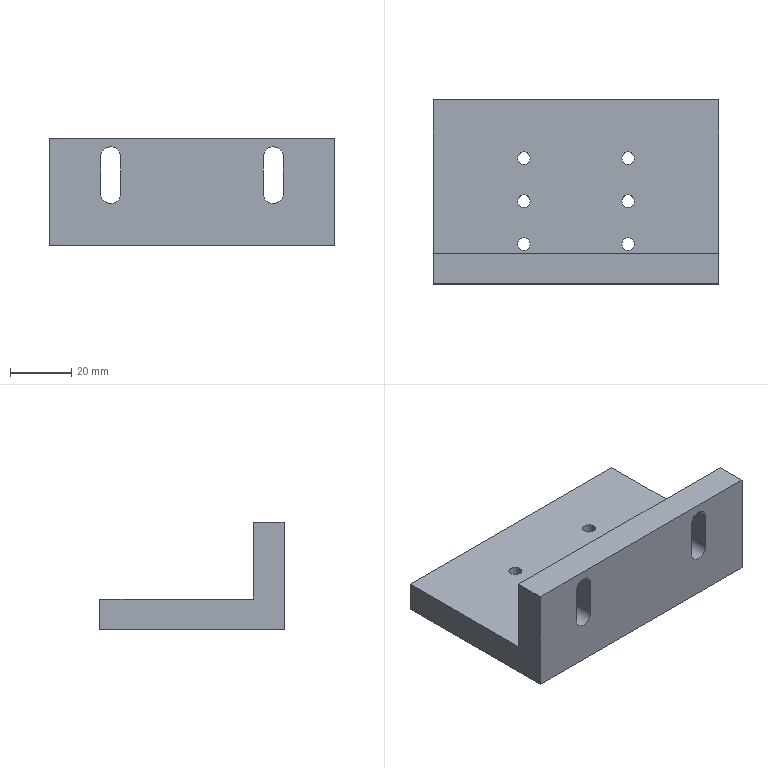Part | NX | 1 solid | 22 faces | box 93 x 60 x 35 mm | volume 76021 mm3 | plane 12 | cylinder 10 | commonest cylinder face diameters 4.134 x6 6.5 x4
STEP:
#1=CARTESIAN_POINT('',(-14.933,-3.,0.));
#2=VERTEX_POINT('',#1);
#3=CARTESIAN_POINT('',(-17.,-3.,0.));
#4=DIRECTION('',(0.,0.,1.));
#5=DIRECTION('',(1.,0.,0.));
#6=AXIS2_PLACEMENT_3D('',#3,#4,#5);
#7=CIRCLE('',#6,2.067);
#8=EDGE_CURVE('',#2,#2,#7,.T.);
#9=ORIENTED_EDGE('',*,*,#8,.T.);
#10=EDGE_LOOP('',(#9));
#11=FACE_BOUND('',#10,.T.);
#12=CARTESIAN_POINT('',(19.067,-3.,0.));
#13=VERTEX_POINT('',#12);
#14=CARTESIAN_POINT('',(17.,-3.,0.));
#15=DIRECTION('',(0.,0.,1.));
#16=DIRECTION('',(1.,0.,0.));
#17=AXIS2_PLACEMENT_3D('',#14,#15,#16);
#18=CIRCLE('',#17,2.067);
#19=EDGE_CURVE('',#13,#13,#18,.T.);
#20=ORIENTED_EDGE('',*,*,#19,.T.);
#21=EDGE_LOOP('',(#20));
#22=FACE_BOUND('',#21,.T.);
#23=CARTESIAN_POINT('',(-14.933,11.,0.));
#24=VERTEX_POINT('',#23);
#25=CARTESIAN_POINT('',(-17.,11.,0.));
#26=DIRECTION('',(0.,0.,1.));
#27=DIRECTION('',(1.,0.,0.));
#28=AXIS2_PLACEMENT_3D('',#25,#26,#27);
#29=CIRCLE('',#28,2.067);
#30=EDGE_CURVE('',#24,#24,#29,.T.);
#31=ORIENTED_EDGE('',*,*,#30,.T.);
#32=EDGE_LOOP('',(#31));
#33=FACE_BOUND('',#32,.T.);
#34=CARTESIAN_POINT('',(19.067,11.,0.));
#35=VERTEX_POINT('',#34);
#36=CARTESIAN_POINT('',(17.,11.,0.));
#37=DIRECTION('',(0.,0.,1.));
#38=DIRECTION('',(1.,0.,0.));
#39=AXIS2_PLACEMENT_3D('',#36,#37,#38);
#40=CIRCLE('',#39,2.067);
#41=EDGE_CURVE('',#35,#35,#40,.T.);
#42=ORIENTED_EDGE('',*,*,#41,.T.);
#43=EDGE_LOOP('',(#42));
#44=FACE_BOUND('',#43,.T.);
#45=CARTESIAN_POINT('',(-14.933,-17.,0.));
#46=VERTEX_POINT('',#45);
#47=CARTESIAN_POINT('',(-17.,-17.,0.));
#48=DIRECTION('',(0.,0.,1.));
#49=DIRECTION('',(1.,0.,0.));
#50=AXIS2_PLACEMENT_3D('',#47,#48,#49);
#51=CIRCLE('',#50,2.067);
#52=EDGE_CURVE('',#46,#46,#51,.T.);
#53=ORIENTED_EDGE('',*,*,#52,.T.);
#54=EDGE_LOOP('',(#53));
#55=FACE_BOUND('',#54,.T.);
#56=CARTESIAN_POINT('',(19.067,-17.,0.));
#57=VERTEX_POINT('',#56);
#58=CARTESIAN_POINT('',(17.,-17.,0.));
#59=DIRECTION('',(0.,0.,1.));
#60=DIRECTION('',(1.,0.,0.));
#61=AXIS2_PLACEMENT_3D('',#58,#59,#60);
#62=CIRCLE('',#61,2.067);
#63=EDGE_CURVE('',#57,#57,#62,.T.);
#64=ORIENTED_EDGE('',*,*,#63,.T.);
#65=EDGE_LOOP('',(#64));
#66=FACE_BOUND('',#65,.T.);
#67=CARTESIAN_POINT('',(46.5,-30.,0.));
#68=VERTEX_POINT('',#67);
#69=CARTESIAN_POINT('',(46.5,30.,0.));
#70=VERTEX_POINT('',#69);
#71=CARTESIAN_POINT('',(46.5,-30.,0.));
#72=DIRECTION('',(0.,1.,0.));
#73=VECTOR('',#72,1000.);
#74=LINE('',#71,#73);
#75=EDGE_CURVE('',#68,#70,#74,.T.);
#76=ORIENTED_EDGE('',*,*,#75,.F.);
#77=CARTESIAN_POINT('',(-46.5,-30.,0.));
#78=VERTEX_POINT('',#77);
#79=CARTESIAN_POINT('',(-46.5,-30.,0.));
#80=DIRECTION('',(1.,0.,0.));
#81=VECTOR('',#80,1000.);
#82=LINE('',#79,#81);
#83=EDGE_CURVE('',#78,#68,#82,.T.);
#84=ORIENTED_EDGE('',*,*,#83,.F.);
#85=CARTESIAN_POINT('',(-46.5,30.,0.));
#86=VERTEX_POINT('',#85);
#87=CARTESIAN_POINT('',(-46.5,30.,0.));
#88=DIRECTION('',(0.,-1.,0.));
#89=VECTOR('',#88,1000.);
#90=LINE('',#87,#89);
#91=EDGE_CURVE('',#86,#78,#90,.T.);
#92=ORIENTED_EDGE('',*,*,#91,.F.);
#93=CARTESIAN_POINT('',(46.5,30.,0.));
#94=DIRECTION('',(-1.,0.,0.));
#95=VECTOR('',#94,1000.);
#96=LINE('',#93,#95);
#97=EDGE_CURVE('',#70,#86,#96,.T.);
#98=ORIENTED_EDGE('',*,*,#97,.F.);
#99=EDGE_LOOP('',(#76,#84,#92,#98));
#100=FACE_BOUND('',#99,.T.);
#101=CARTESIAN_POINT('',(0.,0.,0.));
#102=DIRECTION('',(0.,0.,1.));
#103=DIRECTION('',(1.,0.,0.));
#104=AXIS2_PLACEMENT_3D('',#101,#102,#103);
#105=PLANE('',#104);
#106=ADVANCED_FACE('',(#11,#22,#33,#44,#55,#66,#100),#105,.F.);
#107=ORIENTED_EDGE('',*,*,#75,.T.);
#108=CARTESIAN_POINT('',(46.5,30.,10.));
#109=VERTEX_POINT('',#108);
#110=CARTESIAN_POINT('',(46.5,30.,0.));
#111=DIRECTION('',(0.,0.,1.));
#112=VECTOR('',#111,1000.);
#113=LINE('',#110,#112);
#114=EDGE_CURVE('',#70,#109,#113,.T.);
#115=ORIENTED_EDGE('',*,*,#114,.T.);
#116=CARTESIAN_POINT('',(46.5,-20.,10.));
#117=VERTEX_POINT('',#116);
#118=CARTESIAN_POINT('',(46.5,-30.,10.));
#119=DIRECTION('',(0.,1.,0.));
#120=VECTOR('',#119,1000.);
#121=LINE('',#118,#120);
#122=EDGE_CURVE('',#117,#109,#121,.T.);
#123=ORIENTED_EDGE('',*,*,#122,.F.);
#124=CARTESIAN_POINT('',(46.5,-20.,35.));
#125=VERTEX_POINT('',#124);
#126=CARTESIAN_POINT('',(46.5,-20.,10.));
#127=DIRECTION('',(0.,0.,1.));
#128=VECTOR('',#127,1000.);
#129=LINE('',#126,#128);
#130=EDGE_CURVE('',#117,#125,#129,.T.);
#131=ORIENTED_EDGE('',*,*,#130,.T.);
#132=CARTESIAN_POINT('',(46.5,-30.,35.));
#133=VERTEX_POINT('',#132);
#134=CARTESIAN_POINT('',(46.5,-30.,35.));
#135=DIRECTION('',(0.,1.,0.));
#136=VECTOR('',#135,1000.);
#137=LINE('',#134,#136);
#138=EDGE_CURVE('',#133,#125,#137,.T.);
#139=ORIENTED_EDGE('',*,*,#138,.F.);
#140=CARTESIAN_POINT('',(46.5,-30.,0.));
#141=DIRECTION('',(0.,0.,1.));
#142=VECTOR('',#141,1000.);
#143=LINE('',#140,#142);
#144=EDGE_CURVE('',#68,#133,#143,.T.);
#145=ORIENTED_EDGE('',*,*,#144,.F.);
#146=EDGE_LOOP('',(#107,#115,#123,#131,#139,#145));
#147=FACE_BOUND('',#146,.T.);
#148=CARTESIAN_POINT('',(46.5,-30.,0.));
#149=DIRECTION('',(1.,0.,0.));
#150=DIRECTION('',(0.,1.,0.));
#151=AXIS2_PLACEMENT_3D('',#148,#149,#150);
#152=PLANE('',#151);
#153=ADVANCED_FACE('',(#147),#152,.T.);
#154=ORIENTED_EDGE('',*,*,#97,.T.);
#155=CARTESIAN_POINT('',(-46.5,30.,10.));
#156=VERTEX_POINT('',#155);
#157=CARTESIAN_POINT('',(-46.5,30.,0.));
#158=DIRECTION('',(0.,0.,1.));
#159=VECTOR('',#158,1000.);
#160=LINE('',#157,#159);
#161=EDGE_CURVE('',#86,#156,#160,.T.);
#162=ORIENTED_EDGE('',*,*,#161,.T.);
#163=CARTESIAN_POINT('',(46.5,30.,10.));
#164=DIRECTION('',(-1.,0.,0.));
#165=VECTOR('',#164,1000.);
#166=LINE('',#163,#165);
#167=EDGE_CURVE('',#109,#156,#166,.T.);
#168=ORIENTED_EDGE('',*,*,#167,.F.);
#169=ORIENTED_EDGE('',*,*,#114,.F.);
#170=EDGE_LOOP('',(#154,#162,#168,#169));
#171=FACE_BOUND('',#170,.T.);
#172=CARTESIAN_POINT('',(46.5,30.,0.));
#173=DIRECTION('',(0.,1.,0.));
#174=DIRECTION('',(-1.,0.,0.));
#175=AXIS2_PLACEMENT_3D('',#172,#173,#174);
#176=PLANE('',#175);
#177=ADVANCED_FACE('',(#171),#176,.T.);
#178=ORIENTED_EDGE('',*,*,#91,.T.);
#179=CARTESIAN_POINT('',(-46.5,-30.,35.));
#180=VERTEX_POINT('',#179);
#181=CARTESIAN_POINT('',(-46.5,-30.,0.));
#182=DIRECTION('',(0.,0.,1.));
#183=VECTOR('',#182,1000.);
#184=LINE('',#181,#183);
#185=EDGE_CURVE('',#78,#180,#184,.T.);
#186=ORIENTED_EDGE('',*,*,#185,.T.);
#187=CARTESIAN_POINT('',(-46.5,-20.,35.));
#188=VERTEX_POINT('',#187);
#189=CARTESIAN_POINT('',(-46.5,30.,35.));
#190=DIRECTION('',(0.,-1.,0.));
#191=VECTOR('',#190,1000.);
#192=LINE('',#189,#191);
#193=EDGE_CURVE('',#188,#180,#192,.T.);
#194=ORIENTED_EDGE('',*,*,#193,.F.);
#195=CARTESIAN_POINT('',(-46.5,-20.,10.));
#196=VERTEX_POINT('',#195);
#197=CARTESIAN_POINT('',(-46.5,-20.,10.));
#198=DIRECTION('',(0.,0.,1.));
#199=VECTOR('',#198,1000.);
#200=LINE('',#197,#199);
#201=EDGE_CURVE('',#196,#188,#200,.T.);
#202=ORIENTED_EDGE('',*,*,#201,.F.);
#203=CARTESIAN_POINT('',(-46.5,30.,10.));
#204=DIRECTION('',(0.,-1.,0.));
#205=VECTOR('',#204,1000.);
#206=LINE('',#203,#205);
#207=EDGE_CURVE('',#156,#196,#206,.T.);
#208=ORIENTED_EDGE('',*,*,#207,.F.);
#209=ORIENTED_EDGE('',*,*,#161,.F.);
#210=EDGE_LOOP('',(#178,#186,#194,#202,#208,#209));
#211=FACE_BOUND('',#210,.T.);
#212=CARTESIAN_POINT('',(-46.5,30.,0.));
#213=DIRECTION('',(-1.,0.,0.));
#214=DIRECTION('',(0.,-1.,0.));
#215=AXIS2_PLACEMENT_3D('',#212,#213,#214);
#216=PLANE('',#215);
#217=ADVANCED_FACE('',(#211),#216,.T.);
#218=CARTESIAN_POINT('',(-29.75,-30.,17.));
#219=VERTEX_POINT('',#218);
#220=CARTESIAN_POINT('',(-29.75,-30.,29.));
#221=VERTEX_POINT('',#220);
#222=CARTESIAN_POINT('',(-29.75,-30.,14.5));
#223=DIRECTION('',(0.,0.,1.));
#224=VECTOR('',#223,1000.);
#225=LINE('',#222,#224);
#226=EDGE_CURVE('',#219,#221,#225,.T.);
#227=ORIENTED_EDGE('',*,*,#226,.T.);
#228=CARTESIAN_POINT('',(-23.25,-30.,29.));
#229=VERTEX_POINT('',#228);
#230=CARTESIAN_POINT('',(-26.5,-30.,29.));
#231=DIRECTION('',(0.,1.,0.));
#232=DIRECTION('',(-1.,0.,0.));
#233=AXIS2_PLACEMENT_3D('',#230,#231,#232);
#234=CIRCLE('',#233,3.25);
#235=EDGE_CURVE('',#221,#229,#234,.T.);
#236=ORIENTED_EDGE('',*,*,#235,.T.);
#237=CARTESIAN_POINT('',(-23.25,-30.,17.));
#238=VERTEX_POINT('',#237);
#239=CARTESIAN_POINT('',(-23.25,-30.,8.5));
#240=DIRECTION('',(0.,0.,-1.));
#241=VECTOR('',#240,1000.);
#242=LINE('',#239,#241);
#243=EDGE_CURVE('',#229,#238,#242,.T.);
#244=ORIENTED_EDGE('',*,*,#243,.T.);
#245=CARTESIAN_POINT('',(-26.5,-30.,17.));
#246=DIRECTION('',(0.,1.,0.));
#247=DIRECTION('',(1.,0.,0.));
#248=AXIS2_PLACEMENT_3D('',#245,#246,#247);
#249=CIRCLE('',#248,3.25);
#250=EDGE_CURVE('',#238,#219,#249,.T.);
#251=ORIENTED_EDGE('',*,*,#250,.T.);
#252=EDGE_LOOP('',(#227,#236,#244,#251));
#253=FACE_BOUND('',#252,.T.);
#254=CARTESIAN_POINT('',(23.25,-30.,17.));
#255=VERTEX_POINT('',#254);
#256=CARTESIAN_POINT('',(23.25,-30.,29.));
#257=VERTEX_POINT('',#256);
#258=CARTESIAN_POINT('',(23.25,-30.,14.5));
#259=DIRECTION('',(0.,0.,1.));
#260=VECTOR('',#259,1000.);
#261=LINE('',#258,#260);
#262=EDGE_CURVE('',#255,#257,#261,.T.);
#263=ORIENTED_EDGE('',*,*,#262,.T.);
#264=CARTESIAN_POINT('',(29.75,-30.,29.));
#265=VERTEX_POINT('',#264);
#266=CARTESIAN_POINT('',(26.5,-30.,29.));
#267=DIRECTION('',(0.,1.,0.));
#268=DIRECTION('',(-1.,0.,0.));
#269=AXIS2_PLACEMENT_3D('',#266,#267,#268);
#270=CIRCLE('',#269,3.25);
#271=EDGE_CURVE('',#257,#265,#270,.T.);
#272=ORIENTED_EDGE('',*,*,#271,.T.);
#273=CARTESIAN_POINT('',(29.75,-30.,17.));
#274=VERTEX_POINT('',#273);
#275=CARTESIAN_POINT('',(29.75,-30.,8.5));
#276=DIRECTION('',(0.,0.,-1.));
#277=VECTOR('',#276,1000.);
#278=LINE('',#275,#277);
#279=EDGE_CURVE('',#265,#274,#278,.T.);
#280=ORIENTED_EDGE('',*,*,#279,.T.);
#281=CARTESIAN_POINT('',(26.5,-30.,17.));
#282=DIRECTION('',(0.,1.,0.));
#283=DIRECTION('',(1.,0.,0.));
#284=AXIS2_PLACEMENT_3D('',#281,#282,#283);
#285=CIRCLE('',#284,3.25);
#286=EDGE_CURVE('',#274,#255,#285,.T.);
#287=ORIENTED_EDGE('',*,*,#286,.T.);
#288=EDGE_LOOP('',(#263,#272,#280,#287));
#289=FACE_BOUND('',#288,.T.);
#290=ORIENTED_EDGE('',*,*,#83,.T.);
#291=ORIENTED_EDGE('',*,*,#144,.T.);
#292=CARTESIAN_POINT('',(-46.5,-30.,35.));
#293=DIRECTION('',(1.,0.,0.));
#294=VECTOR('',#293,1000.);
#295=LINE('',#292,#294);
#296=EDGE_CURVE('',#180,#133,#295,.T.);
#297=ORIENTED_EDGE('',*,*,#296,.F.);
#298=ORIENTED_EDGE('',*,*,#185,.F.);
#299=EDGE_LOOP('',(#290,#291,#297,#298));
#300=FACE_BOUND('',#299,.T.);
#301=CARTESIAN_POINT('',(-46.5,-30.,0.));
#302=DIRECTION('',(0.,-1.,0.));
#303=DIRECTION('',(1.,0.,0.));
#304=AXIS2_PLACEMENT_3D('',#301,#302,#303);
#305=PLANE('',#304);
#306=ADVANCED_FACE('',(#253,#289,#300),#305,.T.);
#307=CARTESIAN_POINT('',(-14.933,-3.,10.));
#308=VERTEX_POINT('',#307);
#309=CARTESIAN_POINT('',(-17.,-3.,10.));
#310=DIRECTION('',(0.,0.,-1.));
#311=DIRECTION('',(1.,0.,0.));
#312=AXIS2_PLACEMENT_3D('',#309,#310,#311);
#313=CIRCLE('',#312,2.067);
#314=EDGE_CURVE('',#308,#308,#313,.T.);
#315=ORIENTED_EDGE('',*,*,#314,.T.);
#316=EDGE_LOOP('',(#315));
#317=FACE_BOUND('',#316,.T.);
#318=CARTESIAN_POINT('',(19.067,-3.,10.));
#319=VERTEX_POINT('',#318);
#320=CARTESIAN_POINT('',(17.,-3.,10.));
#321=DIRECTION('',(0.,0.,-1.));
#322=DIRECTION('',(1.,0.,0.));
#323=AXIS2_PLACEMENT_3D('',#320,#321,#322);
#324=CIRCLE('',#323,2.067);
#325=EDGE_CURVE('',#319,#319,#324,.T.);
#326=ORIENTED_EDGE('',*,*,#325,.T.);
#327=EDGE_LOOP('',(#326));
#328=FACE_BOUND('',#327,.T.);
#329=CARTESIAN_POINT('',(-14.933,11.,10.));
#330=VERTEX_POINT('',#329);
#331=CARTESIAN_POINT('',(-17.,11.,10.));
#332=DIRECTION('',(0.,0.,-1.));
#333=DIRECTION('',(1.,0.,0.));
#334=AXIS2_PLACEMENT_3D('',#331,#332,#333);
#335=CIRCLE('',#334,2.067);
#336=EDGE_CURVE('',#330,#330,#335,.T.);
#337=ORIENTED_EDGE('',*,*,#336,.T.);
#338=EDGE_LOOP('',(#337));
#339=FACE_BOUND('',#338,.T.);
#340=CARTESIAN_POINT('',(19.067,11.,10.));
#341=VERTEX_POINT('',#340);
#342=CARTESIAN_POINT('',(17.,11.,10.));
#343=DIRECTION('',(0.,0.,-1.));
#344=DIRECTION('',(1.,0.,0.));
#345=AXIS2_PLACEMENT_3D('',#342,#343,#344);
#346=CIRCLE('',#345,2.067);
#347=EDGE_CURVE('',#341,#341,#346,.T.);
#348=ORIENTED_EDGE('',*,*,#347,.T.);
#349=EDGE_LOOP('',(#348));
#350=FACE_BOUND('',#349,.T.);
#351=CARTESIAN_POINT('',(-14.933,-17.,10.));
#352=VERTEX_POINT('',#351);
#353=CARTESIAN_POINT('',(-17.,-17.,10.));
#354=DIRECTION('',(0.,0.,-1.));
#355=DIRECTION('',(1.,0.,0.));
#356=AXIS2_PLACEMENT_3D('',#353,#354,#355);
#357=CIRCLE('',#356,2.067);
#358=EDGE_CURVE('',#352,#352,#357,.T.);
#359=ORIENTED_EDGE('',*,*,#358,.T.);
#360=EDGE_LOOP('',(#359));
#361=FACE_BOUND('',#360,.T.);
#362=CARTESIAN_POINT('',(19.067,-17.,10.));
#363=VERTEX_POINT('',#362);
#364=CARTESIAN_POINT('',(17.,-17.,10.));
#365=DIRECTION('',(0.,0.,-1.));
#366=DIRECTION('',(1.,0.,0.));
#367=AXIS2_PLACEMENT_3D('',#364,#365,#366);
#368=CIRCLE('',#367,2.067);
#369=EDGE_CURVE('',#363,#363,#368,.T.);
#370=ORIENTED_EDGE('',*,*,#369,.T.);
#371=EDGE_LOOP('',(#370));
#372=FACE_BOUND('',#371,.T.);
#373=CARTESIAN_POINT('',(23.25,-20.,10.));
#374=DIRECTION('',(1.,0.,0.));
#375=VECTOR('',#374,1000.);
#376=LINE('',#373,#375);
#377=EDGE_CURVE('',#196,#117,#376,.T.);
#378=ORIENTED_EDGE('',*,*,#377,.T.);
#379=ORIENTED_EDGE('',*,*,#122,.T.);
#380=ORIENTED_EDGE('',*,*,#167,.T.);
#381=ORIENTED_EDGE('',*,*,#207,.T.);
#382=EDGE_LOOP('',(#378,#379,#380,#381));
#383=FACE_BOUND('',#382,.T.);
#384=CARTESIAN_POINT('',(0.,0.,10.));
#385=DIRECTION('',(0.,0.,1.));
#386=DIRECTION('',(1.,0.,0.));
#387=AXIS2_PLACEMENT_3D('',#384,#385,#386);
#388=PLANE('',#387);
#389=ADVANCED_FACE('',(#317,#328,#339,#350,#361,#372,#383),#388,.T.);
#390=ORIENTED_EDGE('',*,*,#138,.T.);
#391=CARTESIAN_POINT('',(46.5,-20.,35.));
#392=DIRECTION('',(-1.,0.,0.));
#393=VECTOR('',#392,1000.);
#394=LINE('',#391,#393);
#395=EDGE_CURVE('',#125,#188,#394,.T.);
#396=ORIENTED_EDGE('',*,*,#395,.T.);
#397=ORIENTED_EDGE('',*,*,#193,.T.);
#398=ORIENTED_EDGE('',*,*,#296,.T.);
#399=EDGE_LOOP('',(#390,#396,#397,#398));
#400=FACE_BOUND('',#399,.T.);
#401=CARTESIAN_POINT('',(0.,-25.,35.));
#402=DIRECTION('',(0.,0.,1.));
#403=DIRECTION('',(1.,0.,0.));
#404=AXIS2_PLACEMENT_3D('',#401,#402,#403);
#405=PLANE('',#404);
#406=ADVANCED_FACE('',(#400),#405,.T.);
#407=CARTESIAN_POINT('',(-29.75,-20.,29.));
#408=VERTEX_POINT('',#407);
#409=CARTESIAN_POINT('',(-29.75,-20.,17.));
#410=VERTEX_POINT('',#409);
#411=CARTESIAN_POINT('',(-29.75,-20.,19.5));
#412=DIRECTION('',(0.,0.,-1.));
#413=VECTOR('',#412,1000.);
#414=LINE('',#411,#413);
#415=EDGE_CURVE('',#408,#410,#414,.T.);
#416=ORIENTED_EDGE('',*,*,#415,.T.);
#417=CARTESIAN_POINT('',(-23.25,-20.,17.));
#418=VERTEX_POINT('',#417);
#419=CARTESIAN_POINT('',(-26.5,-20.,17.));
#420=DIRECTION('',(0.,-1.,0.));
#421=DIRECTION('',(1.,0.,0.));
#422=AXIS2_PLACEMENT_3D('',#419,#420,#421);
#423=CIRCLE('',#422,3.25);
#424=EDGE_CURVE('',#410,#418,#423,.T.);
#425=ORIENTED_EDGE('',*,*,#424,.T.);
#426=CARTESIAN_POINT('',(-23.25,-20.,29.));
#427=VERTEX_POINT('',#426);
#428=CARTESIAN_POINT('',(-23.25,-20.,13.5));
#429=DIRECTION('',(0.,0.,1.));
#430=VECTOR('',#429,1000.);
#431=LINE('',#428,#430);
#432=EDGE_CURVE('',#418,#427,#431,.T.);
#433=ORIENTED_EDGE('',*,*,#432,.T.);
#434=CARTESIAN_POINT('',(-26.5,-20.,29.));
#435=DIRECTION('',(0.,-1.,0.));
#436=DIRECTION('',(-1.,0.,0.));
#437=AXIS2_PLACEMENT_3D('',#434,#435,#436);
#438=CIRCLE('',#437,3.25);
#439=EDGE_CURVE('',#427,#408,#438,.T.);
#440=ORIENTED_EDGE('',*,*,#439,.T.);
#441=EDGE_LOOP('',(#416,#425,#433,#440));
#442=FACE_BOUND('',#441,.T.);
#443=CARTESIAN_POINT('',(23.25,-20.,29.));
#444=VERTEX_POINT('',#443);
#445=CARTESIAN_POINT('',(23.25,-20.,17.));
#446=VERTEX_POINT('',#445);
#447=CARTESIAN_POINT('',(23.25,-20.,19.5));
#448=DIRECTION('',(0.,0.,-1.));
#449=VECTOR('',#448,1000.);
#450=LINE('',#447,#449);
#451=EDGE_CURVE('',#444,#446,#450,.T.);
#452=ORIENTED_EDGE('',*,*,#451,.T.);
#453=CARTESIAN_POINT('',(29.75,-20.,17.));
#454=VERTEX_POINT('',#453);
#455=CARTESIAN_POINT('',(26.5,-20.,17.));
#456=DIRECTION('',(0.,-1.,0.));
#457=DIRECTION('',(1.,0.,0.));
#458=AXIS2_PLACEMENT_3D('',#455,#456,#457);
#459=CIRCLE('',#458,3.25);
#460=EDGE_CURVE('',#446,#454,#459,.T.);
#461=ORIENTED_EDGE('',*,*,#460,.T.);
#462=CARTESIAN_POINT('',(29.75,-20.,29.));
#463=VERTEX_POINT('',#462);
#464=CARTESIAN_POINT('',(29.75,-20.,13.5));
#465=DIRECTION('',(0.,0.,1.));
#466=VECTOR('',#465,1000.);
#467=LINE('',#464,#466);
#468=EDGE_CURVE('',#454,#463,#467,.T.);
#469=ORIENTED_EDGE('',*,*,#468,.T.);
#470=CARTESIAN_POINT('',(26.5,-20.,29.));
#471=DIRECTION('',(0.,-1.,0.));
#472=DIRECTION('',(-1.,0.,0.));
#473=AXIS2_PLACEMENT_3D('',#470,#471,#472);
#474=CIRCLE('',#473,3.25);
#475=EDGE_CURVE('',#463,#444,#474,.T.);
#476=ORIENTED_EDGE('',*,*,#475,.T.);
#477=EDGE_LOOP('',(#452,#461,#469,#476));
#478=FACE_BOUND('',#477,.T.);
#479=ORIENTED_EDGE('',*,*,#377,.F.);
#480=ORIENTED_EDGE('',*,*,#201,.T.);
#481=ORIENTED_EDGE('',*,*,#395,.F.);
#482=ORIENTED_EDGE('',*,*,#130,.F.);
#483=EDGE_LOOP('',(#479,#480,#481,#482));
#484=FACE_BOUND('',#483,.T.);
#485=CARTESIAN_POINT('',(46.5,-20.,10.));
#486=DIRECTION('',(0.,1.,0.));
#487=DIRECTION('',(-1.,0.,0.));
#488=AXIS2_PLACEMENT_3D('',#485,#486,#487);
#489=PLANE('',#488);
#490=ADVANCED_FACE('',(#442,#478,#484),#489,.T.);
#491=ORIENTED_EDGE('',*,*,#8,.F.);
#492=EDGE_LOOP('',(#491));
#493=FACE_BOUND('',#492,.T.);
#494=ORIENTED_EDGE('',*,*,#314,.F.);
#495=EDGE_LOOP('',(#494));
#496=FACE_BOUND('',#495,.T.);
#497=CARTESIAN_POINT('',(-17.,-3.,-106.078));
#498=DIRECTION('',(0.,0.,1.));
#499=DIRECTION('',(1.,0.,0.));
#500=AXIS2_PLACEMENT_3D('',#497,#498,#499);
#501=CYLINDRICAL_SURFACE('',#500,2.067);
#502=ADVANCED_FACE('',(#493,#496),#501,.F.);
#503=ORIENTED_EDGE('',*,*,#19,.F.);
#504=EDGE_LOOP('',(#503));
#505=FACE_BOUND('',#504,.T.);
#506=ORIENTED_EDGE('',*,*,#325,.F.);
#507=EDGE_LOOP('',(#506));
#508=FACE_BOUND('',#507,.T.);
#509=CARTESIAN_POINT('',(17.,-3.,-106.078));
#510=DIRECTION('',(0.,0.,1.));
#511=DIRECTION('',(1.,0.,0.));
#512=AXIS2_PLACEMENT_3D('',#509,#510,#511);
#513=CYLINDRICAL_SURFACE('',#512,2.067);
#514=ADVANCED_FACE('',(#505,#508),#513,.F.);
#515=ORIENTED_EDGE('',*,*,#30,.F.);
#516=EDGE_LOOP('',(#515));
#517=FACE_BOUND('',#516,.T.);
#518=ORIENTED_EDGE('',*,*,#336,.F.);
#519=EDGE_LOOP('',(#518));
#520=FACE_BOUND('',#519,.T.);
#521=CARTESIAN_POINT('',(-17.,11.,-106.078));
#522=DIRECTION('',(0.,0.,1.));
#523=DIRECTION('',(1.,0.,0.));
#524=AXIS2_PLACEMENT_3D('',#521,#522,#523);
#525=CYLINDRICAL_SURFACE('',#524,2.067);
#526=ADVANCED_FACE('',(#517,#520),#525,.F.);
#527=ORIENTED_EDGE('',*,*,#41,.F.);
#528=EDGE_LOOP('',(#527));
#529=FACE_BOUND('',#528,.T.);
#530=ORIENTED_EDGE('',*,*,#347,.F.);
#531=EDGE_LOOP('',(#530));
#532=FACE_BOUND('',#531,.T.);
#533=CARTESIAN_POINT('',(17.,11.,-106.078));
#534=DIRECTION('',(0.,0.,1.));
#535=DIRECTION('',(1.,0.,0.));
#536=AXIS2_PLACEMENT_3D('',#533,#534,#535);
#537=CYLINDRICAL_SURFACE('',#536,2.067);
#538=ADVANCED_FACE('',(#529,#532),#537,.F.);
#539=ORIENTED_EDGE('',*,*,#52,.F.);
#540=EDGE_LOOP('',(#539));
#541=FACE_BOUND('',#540,.T.);
#542=ORIENTED_EDGE('',*,*,#358,.F.);
#543=EDGE_LOOP('',(#542));
#544=FACE_BOUND('',#543,.T.);
#545=CARTESIAN_POINT('',(-17.,-17.,-106.078));
#546=DIRECTION('',(0.,0.,1.));
#547=DIRECTION('',(1.,0.,0.));
#548=AXIS2_PLACEMENT_3D('',#545,#546,#547);
#549=CYLINDRICAL_SURFACE('',#548,2.067);
#550=ADVANCED_FACE('',(#541,#544),#549,.F.);
#551=ORIENTED_EDGE('',*,*,#63,.F.);
#552=EDGE_LOOP('',(#551));
#553=FACE_BOUND('',#552,.T.);
#554=ORIENTED_EDGE('',*,*,#369,.F.);
#555=EDGE_LOOP('',(#554));
#556=FACE_BOUND('',#555,.T.);
#557=CARTESIAN_POINT('',(17.,-17.,-106.078));
#558=DIRECTION('',(0.,0.,1.));
#559=DIRECTION('',(1.,0.,0.));
#560=AXIS2_PLACEMENT_3D('',#557,#558,#559);
#561=CYLINDRICAL_SURFACE('',#560,2.067);
#562=ADVANCED_FACE('',(#553,#556),#561,.F.);
#563=ORIENTED_EDGE('',*,*,#235,.F.);
#564=CARTESIAN_POINT('',(-29.75,-20.,29.));
#565=DIRECTION('',(0.,-1.,0.));
#566=VECTOR('',#565,1000.);
#567=LINE('',#564,#566);
#568=EDGE_CURVE('',#408,#221,#567,.T.);
#569=ORIENTED_EDGE('',*,*,#568,.F.);
#570=ORIENTED_EDGE('',*,*,#439,.F.);
#571=CARTESIAN_POINT('',(-23.25,-20.,29.));
#572=DIRECTION('',(0.,-1.,0.));
#573=VECTOR('',#572,1000.);
#574=LINE('',#571,#573);
#575=EDGE_CURVE('',#427,#229,#574,.T.);
#576=ORIENTED_EDGE('',*,*,#575,.T.);
#577=EDGE_LOOP('',(#563,#569,#570,#576));
#578=FACE_BOUND('',#577,.T.);
#579=CARTESIAN_POINT('',(-26.5,-20.,29.));
#580=DIRECTION('',(0.,-1.,0.));
#581=DIRECTION('',(-1.,0.,0.));
#582=AXIS2_PLACEMENT_3D('',#579,#580,#581);
#583=CYLINDRICAL_SURFACE('',#582,3.25);
#584=ADVANCED_FACE('',(#578),#583,.F.);
#585=ORIENTED_EDGE('',*,*,#226,.F.);
#586=CARTESIAN_POINT('',(-29.75,-20.,17.));
#587=DIRECTION('',(0.,-1.,0.));
#588=VECTOR('',#587,1000.);
#589=LINE('',#586,#588);
#590=EDGE_CURVE('',#410,#219,#589,.T.);
#591=ORIENTED_EDGE('',*,*,#590,.F.);
#592=ORIENTED_EDGE('',*,*,#415,.F.);
#593=ORIENTED_EDGE('',*,*,#568,.T.);
#594=EDGE_LOOP('',(#585,#591,#592,#593));
#595=FACE_BOUND('',#594,.T.);
#596=CARTESIAN_POINT('',(-29.75,-20.,29.));
#597=DIRECTION('',(-1.,0.,0.));
#598=DIRECTION('',(0.,0.,-1.));
#599=AXIS2_PLACEMENT_3D('',#596,#597,#598);
#600=PLANE('',#599);
#601=ADVANCED_FACE('',(#595),#600,.F.);
#602=ORIENTED_EDGE('',*,*,#250,.F.);
#603=CARTESIAN_POINT('',(-23.25,-20.,17.));
#604=DIRECTION('',(0.,-1.,0.));
#605=VECTOR('',#604,1000.);
#606=LINE('',#603,#605);
#607=EDGE_CURVE('',#418,#238,#606,.T.);
#608=ORIENTED_EDGE('',*,*,#607,.F.);
#609=ORIENTED_EDGE('',*,*,#424,.F.);
#610=ORIENTED_EDGE('',*,*,#590,.T.);
#611=EDGE_LOOP('',(#602,#608,#609,#610));
#612=FACE_BOUND('',#611,.T.);
#613=CARTESIAN_POINT('',(-26.5,-20.,17.));
#614=DIRECTION('',(0.,-1.,0.));
#615=DIRECTION('',(1.,0.,0.));
#616=AXIS2_PLACEMENT_3D('',#613,#614,#615);
#617=CYLINDRICAL_SURFACE('',#616,3.25);
#618=ADVANCED_FACE('',(#612),#617,.F.);
#619=ORIENTED_EDGE('',*,*,#243,.F.);
#620=ORIENTED_EDGE('',*,*,#575,.F.);
#621=ORIENTED_EDGE('',*,*,#432,.F.);
#622=ORIENTED_EDGE('',*,*,#607,.T.);
#623=EDGE_LOOP('',(#619,#620,#621,#622));
#624=FACE_BOUND('',#623,.T.);
#625=CARTESIAN_POINT('',(-23.25,-20.,17.));
#626=DIRECTION('',(1.,0.,0.));
#627=DIRECTION('',(0.,0.,1.));
#628=AXIS2_PLACEMENT_3D('',#625,#626,#627);
#629=PLANE('',#628);
#630=ADVANCED_FACE('',(#624),#629,.F.);
#631=ORIENTED_EDGE('',*,*,#271,.F.);
#632=CARTESIAN_POINT('',(23.25,-20.,29.));
#633=DIRECTION('',(0.,-1.,0.));
#634=VECTOR('',#633,1000.);
#635=LINE('',#632,#634);
#636=EDGE_CURVE('',#444,#257,#635,.T.);
#637=ORIENTED_EDGE('',*,*,#636,.F.);
#638=ORIENTED_EDGE('',*,*,#475,.F.);
#639=CARTESIAN_POINT('',(29.75,-20.,29.));
#640=DIRECTION('',(0.,-1.,0.));
#641=VECTOR('',#640,1000.);
#642=LINE('',#639,#641);
#643=EDGE_CURVE('',#463,#265,#642,.T.);
#644=ORIENTED_EDGE('',*,*,#643,.T.);
#645=EDGE_LOOP('',(#631,#637,#638,#644));
#646=FACE_BOUND('',#645,.T.);
#647=CARTESIAN_POINT('',(26.5,-20.,29.));
#648=DIRECTION('',(0.,-1.,0.));
#649=DIRECTION('',(-1.,0.,0.));
#650=AXIS2_PLACEMENT_3D('',#647,#648,#649);
#651=CYLINDRICAL_SURFACE('',#650,3.25);
#652=ADVANCED_FACE('',(#646),#651,.F.);
#653=ORIENTED_EDGE('',*,*,#262,.F.);
#654=CARTESIAN_POINT('',(23.25,-20.,17.));
#655=DIRECTION('',(0.,-1.,0.));
#656=VECTOR('',#655,1000.);
#657=LINE('',#654,#656);
#658=EDGE_CURVE('',#446,#255,#657,.T.);
#659=ORIENTED_EDGE('',*,*,#658,.F.);
#660=ORIENTED_EDGE('',*,*,#451,.F.);
#661=ORIENTED_EDGE('',*,*,#636,.T.);
#662=EDGE_LOOP('',(#653,#659,#660,#661));
#663=FACE_BOUND('',#662,.T.);
#664=CARTESIAN_POINT('',(23.25,-20.,29.));
#665=DIRECTION('',(-1.,0.,0.));
#666=DIRECTION('',(0.,0.,-1.));
#667=AXIS2_PLACEMENT_3D('',#664,#665,#666);
#668=PLANE('',#667);
#669=ADVANCED_FACE('',(#663),#668,.F.);
#670=ORIENTED_EDGE('',*,*,#286,.F.);
#671=CARTESIAN_POINT('',(29.75,-20.,17.));
#672=DIRECTION('',(0.,-1.,0.));
#673=VECTOR('',#672,1000.);
#674=LINE('',#671,#673);
#675=EDGE_CURVE('',#454,#274,#674,.T.);
#676=ORIENTED_EDGE('',*,*,#675,.F.);
#677=ORIENTED_EDGE('',*,*,#460,.F.);
#678=ORIENTED_EDGE('',*,*,#658,.T.);
#679=EDGE_LOOP('',(#670,#676,#677,#678));
#680=FACE_BOUND('',#679,.T.);
#681=CARTESIAN_POINT('',(26.5,-20.,17.));
#682=DIRECTION('',(0.,-1.,0.));
#683=DIRECTION('',(1.,0.,0.));
#684=AXIS2_PLACEMENT_3D('',#681,#682,#683);
#685=CYLINDRICAL_SURFACE('',#684,3.25);
#686=ADVANCED_FACE('',(#680),#685,.F.);
#687=ORIENTED_EDGE('',*,*,#279,.F.);
#688=ORIENTED_EDGE('',*,*,#643,.F.);
#689=ORIENTED_EDGE('',*,*,#468,.F.);
#690=ORIENTED_EDGE('',*,*,#675,.T.);
#691=EDGE_LOOP('',(#687,#688,#689,#690));
#692=FACE_BOUND('',#691,.T.);
#693=CARTESIAN_POINT('',(29.75,-20.,17.));
#694=DIRECTION('',(1.,0.,0.));
#695=DIRECTION('',(0.,0.,1.));
#696=AXIS2_PLACEMENT_3D('',#693,#694,#695);
#697=PLANE('',#696);
#698=ADVANCED_FACE('',(#692),#697,.F.);
#699=CLOSED_SHELL('',(#106,#153,#177,#217,#306,#389,#406,#490,#502,#514,#526,#538,#550,#562,#584,#601,#618,#630,#652,#669,#686,#698));
#700=MANIFOLD_SOLID_BREP('',#699);
#701=(LENGTH_UNIT()NAMED_UNIT(*)SI_UNIT(.MILLI.,.METRE.));
#702=UNCERTAINTY_MEASURE_WITH_UNIT(LENGTH_MEASURE(0.00001),#701,'','');
#703=(NAMED_UNIT(*)PLANE_ANGLE_UNIT()SI_UNIT($,.RADIAN.));
#704=(NAMED_UNIT(*)SI_UNIT($,.STERADIAN.)SOLID_ANGLE_UNIT());
#705=(GEOMETRIC_REPRESENTATION_CONTEXT(3)GLOBAL_UNCERTAINTY_ASSIGNED_CONTEXT((#702))GLOBAL_UNIT_ASSIGNED_CONTEXT((#701,#703,#704))REPRESENTATION_CONTEXT('',''));
#706=ADVANCED_BREP_SHAPE_REPRESENTATION('',(#700),#705);